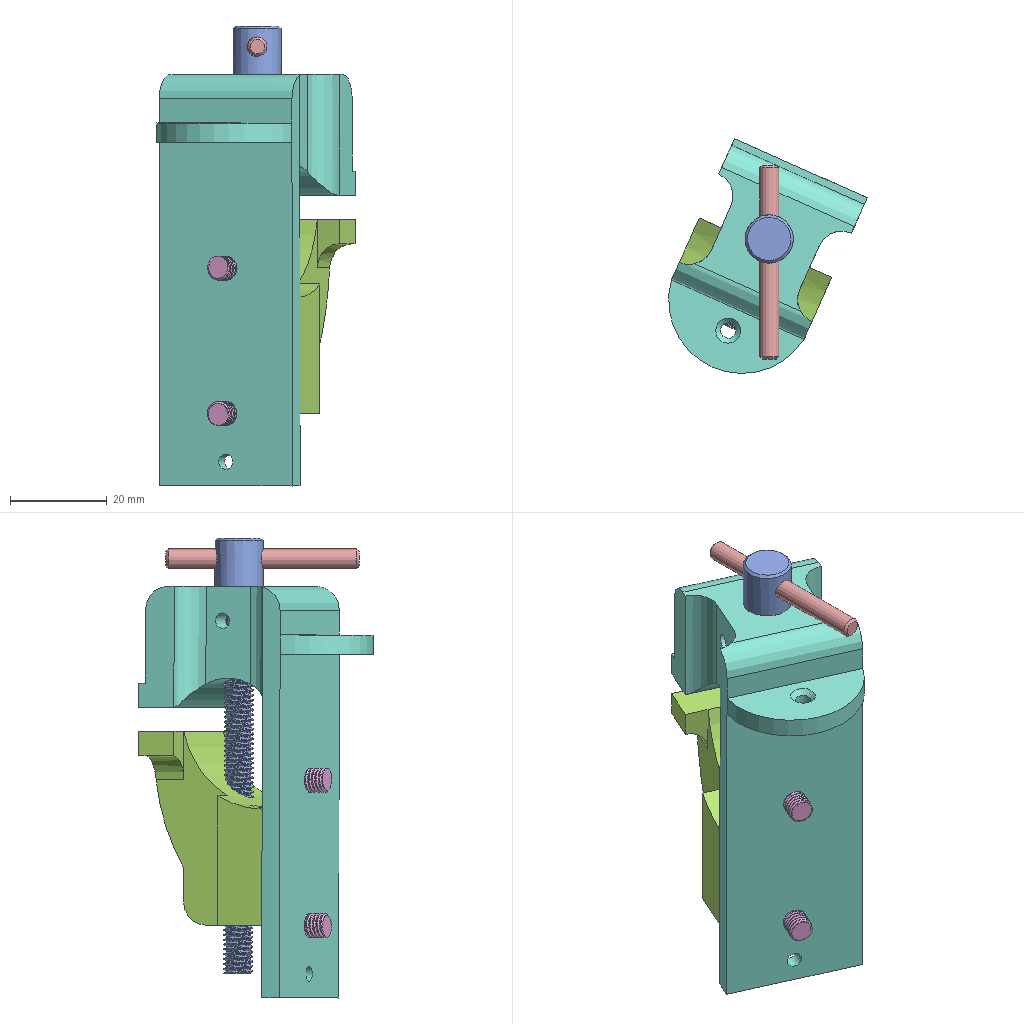Assembly | NX | 5 different items | 6 placed | box 41 x 49 x 95 mm
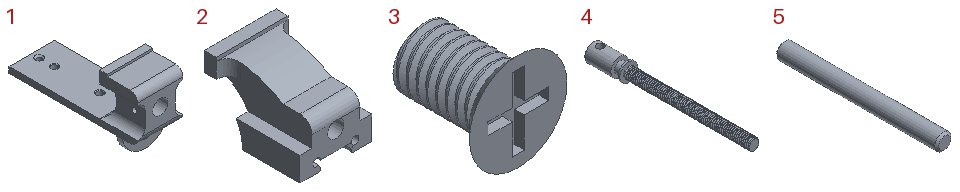Parts list (item | quantity | size | volume | features):
1 | x1 | 30 x 85 x 45 mm | 23577 mm3 | features SKETCH 12, EXTRUDE 11, Linear Dimension 2, SIMPLE HOLE 2, SYMBOLIC_THREAD 2, BLEND 1, CHAMFER 1, DATUM_CSYS 1, HOLE PACKAGE 1
2 | x1 | 30 x 40 x 28 mm | 14530 mm3 | features SKETCH 9, EXTRUDE 8, BLEND 3, DATUM_CSYS 1, HOLE PACKAGE 1, SIMPLE HOLE 1, SYMBOLIC_THREAD 1
3 | x2 | 8 x 8 x 8 mm | 147.132 mm3 | features EXTRUDE 3, SKETCH 3, CHAMFER 1, DATUM_CSYS 1, THREADS 1, UNITE 1
4 | x1 | 10 x 90 x 10 mm | 2885 mm3 | features EXTRUDE 5, SKETCH 4, LINE 2, UNITE 2, CHAMFER 1, DATUM_CSYS 1, INTERSECTION_CURVES 1, THREADS 1
5 | x1 | 4 x 40 x 4 mm | 499.775 mm3 | features CHAMFER 2, DATUM_CSYS 1, EXTRUDE 1, SKETCH 1
Mates (type | each side: item.copy, entity, surface, feature):
Distance | 2.1 face plane Extrude(1) | 1.1 face plane Extrude(3)
Touch | 2.1 face plane Extrude(1) | 1.1 face plane Extrude(3)
Distance | 1.1 face plane Extrude(1) | 4.1 face plane Extrude(1)
Distance | 5.1 | 4.1 ellipse